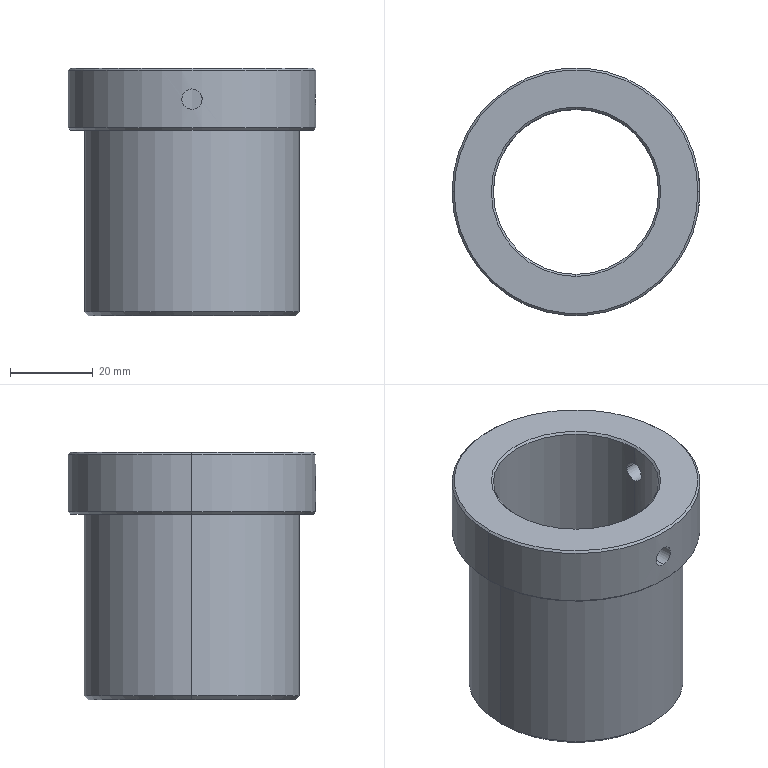Part | STEP file | Coil positioning adjuster | 1 solid | 23 faces | box 60 x 60 x 60 mm | volume 62041 mm3 | cylinder 10 | cone 10 | plane 3 | commonest cylinder face diameters 4.917 x4 40 x2 52 x2 60 x2